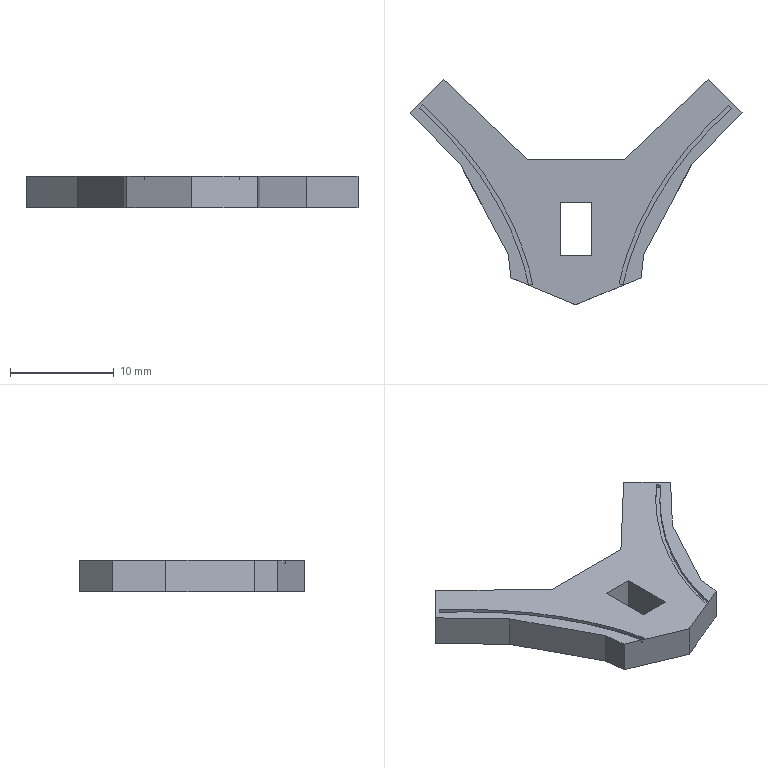Part | SolidWorks | features BaseBody 1 | 1 solid | 29 faces | box 31.951 x 21.72 x 3 mm | volume 821.926 mm3 | plane 25 | spline 4
STEP:
#1=CARTESIAN_POINT('',(13.317,21.551,1.2));
#2=VERTEX_POINT('',#1);
#3=CARTESIAN_POINT('',(2.742,4.389,1.2));
#4=VERTEX_POINT('',#3);
#5=CARTESIAN_POINT('',(13.317,21.551,1.2));
#6=CARTESIAN_POINT('',(10.685,19.267,1.2));
#7=CARTESIAN_POINT('',(4.586,13.173,1.2));
#8=CARTESIAN_POINT('',(2.742,4.389,1.2));
#9=B_SPLINE_CURVE_WITH_KNOTS('',3,(#5,#6,#7,#8),.UNSPECIFIED.,.F.,.F.,(4,4),(0.211,0.9451),.UNSPECIFIED.);
#10=EDGE_CURVE('',#2,#4,#9,.T.);
#11=ORIENTED_EDGE('',*,*,#10,.T.);
#12=CARTESIAN_POINT('',(3.133,4.307,1.2));
#13=VERTEX_POINT('',#12);
#14=CARTESIAN_POINT('',(3.133,4.307,1.2));
#15=DIRECTION('',(-0.9787,0.2054,0.));
#16=VECTOR('',#15,1000.);
#17=LINE('',#14,#16);
#18=EDGE_CURVE('',#13,#4,#17,.T.);
#19=ORIENTED_EDGE('',*,*,#18,.F.);
#20=CARTESIAN_POINT('',(13.579,21.248,1.2));
#21=VERTEX_POINT('',#20);
#22=CARTESIAN_POINT('',(13.579,21.248,1.2));
#23=CARTESIAN_POINT('',(12.281,20.122,1.2));
#24=CARTESIAN_POINT('',(10.119,18.048,1.2));
#25=CARTESIAN_POINT('',(5.999,12.301,1.2));
#26=CARTESIAN_POINT('',(4.041,8.63,1.2));
#27=CARTESIAN_POINT('',(3.133,4.307,1.2));
#28=B_SPLINE_CURVE_WITH_KNOTS('',3,(#22,#23,#24,#25,#26,#27),.UNSPECIFIED.,.F.,.F.,(4,2,4),(0.,0.5,1.),.UNSPECIFIED.);
#29=EDGE_CURVE('',#21,#13,#28,.T.);
#30=ORIENTED_EDGE('',*,*,#29,.F.);
#31=CARTESIAN_POINT('',(13.317,21.551,1.2));
#32=DIRECTION('',(0.6554,-0.7553,0.));
#33=VECTOR('',#32,1000.);
#34=LINE('',#31,#33);
#35=EDGE_CURVE('',#2,#21,#34,.T.);
#36=ORIENTED_EDGE('',*,*,#35,.F.);
#37=EDGE_LOOP('',(#11,#19,#30,#36));
#38=FACE_OUTER_BOUND('',#37,.T.);
#39=CARTESIAN_POINT('',(7.734,15.408,1.2));
#40=DIRECTION('',(0.,0.,-1.));
#41=DIRECTION('',(0.,-1.,0.));
#42=AXIS2_PLACEMENT_3D('',#39,#40,#41);
#43=PLANE('',#42);
#44=ADVANCED_FACE('',(#38),#43,.F.);
#45=CARTESIAN_POINT('',(3.133,4.307,1.5));
#46=VERTEX_POINT('',#45);
#47=CARTESIAN_POINT('',(2.742,4.389,1.5));
#48=VERTEX_POINT('',#47);
#49=CARTESIAN_POINT('',(3.133,4.307,1.5));
#50=DIRECTION('',(-0.9787,0.2054,0.));
#51=VECTOR('',#50,1000.);
#52=LINE('',#49,#51);
#53=EDGE_CURVE('',#46,#48,#52,.T.);
#54=ORIENTED_EDGE('',*,*,#53,.F.);
#55=CARTESIAN_POINT('',(3.133,4.307,1.2));
#56=DIRECTION('',(0.,0.,1.));
#57=VECTOR('',#56,1000.);
#58=LINE('',#55,#57);
#59=EDGE_CURVE('',#13,#46,#58,.T.);
#60=ORIENTED_EDGE('',*,*,#59,.F.);
#61=ORIENTED_EDGE('',*,*,#18,.T.);
#62=CARTESIAN_POINT('',(2.742,4.389,1.2));
#63=DIRECTION('',(0.,0.,1.));
#64=VECTOR('',#63,1000.);
#65=LINE('',#62,#64);
#66=EDGE_CURVE('',#4,#48,#65,.T.);
#67=ORIENTED_EDGE('',*,*,#66,.T.);
#68=EDGE_LOOP('',(#54,#60,#61,#67));
#69=FACE_OUTER_BOUND('',#68,.T.);
#70=CARTESIAN_POINT('',(3.133,4.307,1.2));
#71=DIRECTION('',(0.2054,0.9787,0.));
#72=DIRECTION('',(0.,0.,-1.));
#73=AXIS2_PLACEMENT_3D('',#70,#71,#72);
#74=PLANE('',#73);
#75=ADVANCED_FACE('',(#69),#74,.T.);
#76=CARTESIAN_POINT('',(13.579,21.248,1.5));
#77=VERTEX_POINT('',#76);
#78=CARTESIAN_POINT('',(13.579,21.248,1.5));
#79=CARTESIAN_POINT('',(12.281,20.122,1.5));
#80=CARTESIAN_POINT('',(10.119,18.048,1.5));
#81=CARTESIAN_POINT('',(5.999,12.301,1.5));
#82=CARTESIAN_POINT('',(4.041,8.63,1.5));
#83=CARTESIAN_POINT('',(3.133,4.307,1.5));
#84=B_SPLINE_CURVE_WITH_KNOTS('',3,(#78,#79,#80,#81,#82,#83),.UNSPECIFIED.,.F.,.F.,(4,2,4),(0.,0.5,1.),.UNSPECIFIED.);
#85=EDGE_CURVE('',#77,#46,#84,.T.);
#86=ORIENTED_EDGE('',*,*,#85,.F.);
#87=CARTESIAN_POINT('',(13.579,21.248,1.2));
#88=DIRECTION('',(0.,0.,1.));
#89=VECTOR('',#88,1000.);
#90=LINE('',#87,#89);
#91=EDGE_CURVE('',#21,#77,#90,.T.);
#92=ORIENTED_EDGE('',*,*,#91,.F.);
#93=ORIENTED_EDGE('',*,*,#29,.T.);
#94=ORIENTED_EDGE('',*,*,#59,.T.);
#95=EDGE_LOOP('',(#86,#92,#93,#94));
#96=FACE_OUTER_BOUND('',#95,.T.);
#97=CARTESIAN_POINT('',(13.579,21.248,1.2));
#98=CARTESIAN_POINT('',(13.579,21.248,1.5));
#99=CARTESIAN_POINT('',(12.281,20.122,1.2));
#100=CARTESIAN_POINT('',(12.281,20.122,1.5));
#101=CARTESIAN_POINT('',(10.119,18.048,1.2));
#102=CARTESIAN_POINT('',(10.119,18.048,1.5));
#103=CARTESIAN_POINT('',(5.999,12.301,1.2));
#104=CARTESIAN_POINT('',(5.999,12.301,1.5));
#105=CARTESIAN_POINT('',(4.041,8.63,1.2));
#106=CARTESIAN_POINT('',(4.041,8.63,1.5));
#107=CARTESIAN_POINT('',(3.133,4.307,1.2));
#108=CARTESIAN_POINT('',(3.133,4.307,1.5));
#109=B_SPLINE_SURFACE_WITH_KNOTS('',3,1,((#97,#98),(#99,#100),(#101,#102),(#103,#104),(#105,#106),(#107,#108)),.UNSPECIFIED.,.F.,.F.,.F.,(4,2,4),(2,2),(0.,0.5,1.),(0.,1.),.UNSPECIFIED.);
#110=ADVANCED_FACE('',(#96),#109,.T.);
#111=CARTESIAN_POINT('',(13.317,21.551,1.5));
#112=VERTEX_POINT('',#111);
#113=CARTESIAN_POINT('',(13.317,21.551,1.5));
#114=DIRECTION('',(0.6554,-0.7553,0.));
#115=VECTOR('',#114,1000.);
#116=LINE('',#113,#115);
#117=EDGE_CURVE('',#112,#77,#116,.T.);
#118=ORIENTED_EDGE('',*,*,#117,.F.);
#119=CARTESIAN_POINT('',(13.317,21.551,1.2));
#120=DIRECTION('',(0.,0.,1.));
#121=VECTOR('',#120,1000.);
#122=LINE('',#119,#121);
#123=EDGE_CURVE('',#2,#112,#122,.T.);
#124=ORIENTED_EDGE('',*,*,#123,.F.);
#125=ORIENTED_EDGE('',*,*,#35,.T.);
#126=ORIENTED_EDGE('',*,*,#91,.T.);
#127=EDGE_LOOP('',(#118,#124,#125,#126));
#128=FACE_OUTER_BOUND('',#127,.T.);
#129=CARTESIAN_POINT('',(13.317,21.551,1.2));
#130=DIRECTION('',(-0.7553,-0.6554,0.));
#131=DIRECTION('',(-0.6554,0.7553,0.));
#132=AXIS2_PLACEMENT_3D('',#129,#130,#131);
#133=PLANE('',#132);
#134=ADVANCED_FACE('',(#128),#133,.T.);
#135=CARTESIAN_POINT('',(13.317,21.551,1.5));
#136=CARTESIAN_POINT('',(10.685,19.267,1.5));
#137=CARTESIAN_POINT('',(4.586,13.173,1.5));
#138=CARTESIAN_POINT('',(2.742,4.389,1.5));
#139=B_SPLINE_CURVE_WITH_KNOTS('',3,(#135,#136,#137,#138),.UNSPECIFIED.,.F.,.F.,(4,4),(0.211,0.9451),.UNSPECIFIED.);
#140=EDGE_CURVE('',#112,#48,#139,.T.);
#141=ORIENTED_EDGE('',*,*,#140,.T.);
#142=ORIENTED_EDGE('',*,*,#66,.F.);
#143=ORIENTED_EDGE('',*,*,#10,.F.);
#144=ORIENTED_EDGE('',*,*,#123,.T.);
#145=EDGE_LOOP('',(#141,#142,#143,#144));
#146=FACE_OUTER_BOUND('',#145,.T.);
#147=CARTESIAN_POINT('',(13.317,21.551,1.2));
#148=CARTESIAN_POINT('',(13.317,21.551,1.5));
#149=CARTESIAN_POINT('',(10.685,19.267,1.2));
#150=CARTESIAN_POINT('',(10.685,19.267,1.5));
#151=CARTESIAN_POINT('',(4.586,13.173,1.2));
#152=CARTESIAN_POINT('',(4.586,13.173,1.5));
#153=CARTESIAN_POINT('',(2.742,4.389,1.2));
#154=CARTESIAN_POINT('',(2.742,4.389,1.5));
#155=B_SPLINE_SURFACE_WITH_KNOTS('',3,1,((#147,#148),(#149,#150),(#151,#152),(#153,#154)),.UNSPECIFIED.,.F.,.F.,.F.,(4,4),(2,2),(0.211,0.9451),(0.,1.),.UNSPECIFIED.);
#156=ADVANCED_FACE('',(#146),#155,.F.);
#157=CARTESIAN_POINT('',(-16.223,21.611,1.5));
#158=VERTEX_POINT('',#157);
#159=CARTESIAN_POINT('',(-5.569,4.343,1.5));
#160=VERTEX_POINT('',#159);
#161=CARTESIAN_POINT('',(-16.223,21.611,1.5));
#162=CARTESIAN_POINT('',(-13.627,19.373,1.5));
#163=CARTESIAN_POINT('',(-7.418,13.231,1.5));
#164=CARTESIAN_POINT('',(-5.569,4.343,1.5));
#165=B_SPLINE_CURVE_WITH_KNOTS('',3,(#161,#162,#163,#164),.UNSPECIFIED.,.F.,.F.,(4,4),(0.2044,0.9463),.UNSPECIFIED.);
#166=EDGE_CURVE('',#158,#160,#165,.T.);
#167=ORIENTED_EDGE('',*,*,#166,.F.);
#168=CARTESIAN_POINT('',(-16.223,21.611,1.2));
#169=VERTEX_POINT('',#168);
#170=CARTESIAN_POINT('',(-16.223,21.611,1.2));
#171=DIRECTION('',(0.,0.,1.));
#172=VECTOR('',#171,1000.);
#173=LINE('',#170,#172);
#174=EDGE_CURVE('',#169,#158,#173,.T.);
#175=ORIENTED_EDGE('',*,*,#174,.F.);
#176=CARTESIAN_POINT('',(-5.569,4.343,1.2));
#177=VERTEX_POINT('',#176);
#178=CARTESIAN_POINT('',(-16.223,21.611,1.2));
#179=CARTESIAN_POINT('',(-13.627,19.373,1.2));
#180=CARTESIAN_POINT('',(-7.418,13.231,1.2));
#181=CARTESIAN_POINT('',(-5.569,4.343,1.2));
#182=B_SPLINE_CURVE_WITH_KNOTS('',3,(#178,#179,#180,#181),.UNSPECIFIED.,.F.,.F.,(4,4),(0.2044,0.9463),.UNSPECIFIED.);
#183=EDGE_CURVE('',#169,#177,#182,.T.);
#184=ORIENTED_EDGE('',*,*,#183,.T.);
#185=CARTESIAN_POINT('',(-5.569,4.343,1.2));
#186=DIRECTION('',(0.,0.,1.));
#187=VECTOR('',#186,1000.);
#188=LINE('',#185,#187);
#189=EDGE_CURVE('',#177,#160,#188,.T.);
#190=ORIENTED_EDGE('',*,*,#189,.T.);
#191=EDGE_LOOP('',(#167,#175,#184,#190));
#192=FACE_OUTER_BOUND('',#191,.T.);
#193=CARTESIAN_POINT('',(-16.223,21.611,1.2));
#194=CARTESIAN_POINT('',(-16.223,21.611,1.5));
#195=CARTESIAN_POINT('',(-13.627,19.373,1.2));
#196=CARTESIAN_POINT('',(-13.627,19.373,1.5));
#197=CARTESIAN_POINT('',(-7.418,13.231,1.2));
#198=CARTESIAN_POINT('',(-7.418,13.231,1.5));
#199=CARTESIAN_POINT('',(-5.569,4.343,1.2));
#200=CARTESIAN_POINT('',(-5.569,4.343,1.5));
#201=B_SPLINE_SURFACE_WITH_KNOTS('',3,1,((#193,#194),(#195,#196),(#197,#198),(#199,#200)),.UNSPECIFIED.,.F.,.F.,.F.,(4,4),(2,2),(0.2044,0.9463),(0.,1.),.UNSPECIFIED.);
#202=ADVANCED_FACE('',(#192),#201,.T.);
#203=CARTESIAN_POINT('',(-16.484,21.308,1.5));
#204=VERTEX_POINT('',#203);
#205=CARTESIAN_POINT('',(-16.484,21.308,1.5));
#206=DIRECTION('',(0.6531,0.7573,0.));
#207=VECTOR('',#206,1000.);
#208=LINE('',#205,#207);
#209=EDGE_CURVE('',#204,#158,#208,.T.);
#210=ORIENTED_EDGE('',*,*,#209,.F.);
#211=CARTESIAN_POINT('',(-16.484,21.308,1.2));
#212=VERTEX_POINT('',#211);
#213=CARTESIAN_POINT('',(-16.484,21.308,1.2));
#214=DIRECTION('',(0.,0.,1.));
#215=VECTOR('',#214,1000.);
#216=LINE('',#213,#215);
#217=EDGE_CURVE('',#212,#204,#216,.T.);
#218=ORIENTED_EDGE('',*,*,#217,.F.);
#219=CARTESIAN_POINT('',(-16.484,21.308,1.2));
#220=DIRECTION('',(0.6531,0.7573,0.));
#221=VECTOR('',#220,1000.);
#222=LINE('',#219,#221);
#223=EDGE_CURVE('',#212,#169,#222,.T.);
#224=ORIENTED_EDGE('',*,*,#223,.T.);
#225=ORIENTED_EDGE('',*,*,#174,.T.);
#226=EDGE_LOOP('',(#210,#218,#224,#225));
#227=FACE_OUTER_BOUND('',#226,.T.);
#228=CARTESIAN_POINT('',(-16.484,21.308,1.2));
#229=DIRECTION('',(0.7573,-0.6531,0.));
#230=DIRECTION('',(0.,0.,-1.));
#231=AXIS2_PLACEMENT_3D('',#228,#229,#230);
#232=PLANE('',#231);
#233=ADVANCED_FACE('',(#227),#232,.T.);
#234=CARTESIAN_POINT('',(-5.963,4.271,1.2));
#235=VERTEX_POINT('',#234);
#236=CARTESIAN_POINT('',(-5.947,4.265,1.2));
#237=VERTEX_POINT('',#236);
#238=CARTESIAN_POINT('',(-1.413,2.373,1.2));
#239=DIRECTION('',(0.9229,-0.3851,0.));
#240=VECTOR('',#239,1000.);
#241=LINE('',#238,#240);
#242=EDGE_CURVE('',#235,#237,#241,.T.);
#243=ORIENTED_EDGE('',*,*,#242,.T.);
#244=CARTESIAN_POINT('',(-5.569,4.343,1.2));
#245=DIRECTION('',(-0.979,-0.2036,0.));
#246=VECTOR('',#245,1000.);
#247=LINE('',#244,#246);
#248=EDGE_CURVE('',#177,#237,#247,.T.);
#249=ORIENTED_EDGE('',*,*,#248,.F.);
#250=ORIENTED_EDGE('',*,*,#183,.F.);
#251=ORIENTED_EDGE('',*,*,#223,.F.);
#252=CARTESIAN_POINT('',(-16.484,21.308,1.2));
#253=CARTESIAN_POINT('',(-15.204,20.204,1.2));
#254=CARTESIAN_POINT('',(-13.024,18.13,1.2));
#255=CARTESIAN_POINT('',(-8.858,12.347,1.2));
#256=CARTESIAN_POINT('',(-6.874,8.642,1.2));
#257=CARTESIAN_POINT('',(-5.963,4.271,1.2));
#258=B_SPLINE_CURVE_WITH_KNOTS('',3,(#252,#253,#254,#255,#256,#257),.UNSPECIFIED.,.F.,.F.,(4,2,4),(0.,0.5,0.9996),.UNSPECIFIED.);
#259=EDGE_CURVE('',#212,#235,#258,.T.);
#260=ORIENTED_EDGE('',*,*,#259,.T.);
#261=EDGE_LOOP('',(#243,#249,#250,#251,#260));
#262=FACE_OUTER_BOUND('',#261,.T.);
#263=CARTESIAN_POINT('',(-10.94,15.237,1.2));
#264=DIRECTION('',(0.,0.,1.));
#265=DIRECTION('',(1.,0.,0.));
#266=AXIS2_PLACEMENT_3D('',#263,#264,#265);
#267=PLANE('',#266);
#268=ADVANCED_FACE('',(#262),#267,.T.);
#269=CARTESIAN_POINT('',(-5.947,4.265,1.5));
#270=VERTEX_POINT('',#269);
#271=CARTESIAN_POINT('',(-5.947,4.265,1.5));
#272=DIRECTION('',(0.,0.,1.));
#273=VECTOR('',#272,1000.);
#274=LINE('',#271,#273);
#275=EDGE_CURVE('',#237,#270,#274,.T.);
#276=ORIENTED_EDGE('',*,*,#275,.T.);
#277=CARTESIAN_POINT('',(-5.569,4.343,1.5));
#278=DIRECTION('',(-0.979,-0.2036,0.));
#279=VECTOR('',#278,1000.);
#280=LINE('',#277,#279);
#281=EDGE_CURVE('',#160,#270,#280,.T.);
#282=ORIENTED_EDGE('',*,*,#281,.F.);
#283=ORIENTED_EDGE('',*,*,#189,.F.);
#284=ORIENTED_EDGE('',*,*,#248,.T.);
#285=EDGE_LOOP('',(#276,#282,#283,#284));
#286=FACE_OUTER_BOUND('',#285,.T.);
#287=CARTESIAN_POINT('',(-5.569,4.343,1.2));
#288=DIRECTION('',(-0.2036,0.979,0.));
#289=DIRECTION('',(0.,0.,1.));
#290=AXIS2_PLACEMENT_3D('',#287,#288,#289);
#291=PLANE('',#290);
#292=ADVANCED_FACE('',(#286),#291,.T.);
#293=ORIENTED_EDGE('',*,*,#259,.F.);
#294=ORIENTED_EDGE('',*,*,#217,.T.);
#295=CARTESIAN_POINT('',(-5.963,4.271,1.5));
#296=VERTEX_POINT('',#295);
#297=CARTESIAN_POINT('',(-16.484,21.308,1.5));
#298=CARTESIAN_POINT('',(-15.204,20.204,1.5));
#299=CARTESIAN_POINT('',(-13.024,18.13,1.5));
#300=CARTESIAN_POINT('',(-8.858,12.347,1.5));
#301=CARTESIAN_POINT('',(-6.874,8.642,1.5));
#302=CARTESIAN_POINT('',(-5.963,4.271,1.5));
#303=B_SPLINE_CURVE_WITH_KNOTS('',3,(#297,#298,#299,#300,#301,#302),.UNSPECIFIED.,.F.,.F.,(4,2,4),(0.,0.5,0.9996),.UNSPECIFIED.);
#304=EDGE_CURVE('',#204,#296,#303,.T.);
#305=ORIENTED_EDGE('',*,*,#304,.T.);
#306=CARTESIAN_POINT('',(-5.963,4.271,1.2));
#307=DIRECTION('',(0.,0.,1.));
#308=VECTOR('',#307,1000.);
#309=LINE('',#306,#308);
#310=EDGE_CURVE('',#235,#296,#309,.T.);
#311=ORIENTED_EDGE('',*,*,#310,.F.);
#312=EDGE_LOOP('',(#293,#294,#305,#311));
#313=FACE_OUTER_BOUND('',#312,.T.);
#314=CARTESIAN_POINT('',(-16.484,21.308,1.2));
#315=CARTESIAN_POINT('',(-16.484,21.308,1.5));
#316=CARTESIAN_POINT('',(-15.204,20.204,1.2));
#317=CARTESIAN_POINT('',(-15.204,20.204,1.5));
#318=CARTESIAN_POINT('',(-13.024,18.13,1.2));
#319=CARTESIAN_POINT('',(-13.024,18.13,1.5));
#320=CARTESIAN_POINT('',(-8.858,12.347,1.2));
#321=CARTESIAN_POINT('',(-8.858,12.347,1.5));
#322=CARTESIAN_POINT('',(-6.874,8.642,1.2));
#323=CARTESIAN_POINT('',(-6.874,8.642,1.5));
#324=CARTESIAN_POINT('',(-5.963,4.271,1.2));
#325=CARTESIAN_POINT('',(-5.963,4.271,1.5));
#326=B_SPLINE_SURFACE_WITH_KNOTS('',3,1,((#314,#315),(#316,#317),(#318,#319),(#320,#321),(#322,#323),(#324,#325)),.UNSPECIFIED.,.F.,.F.,.F.,(4,2,4),(2,2),(0.,0.5,0.9996),(0.,1.),.UNSPECIFIED.);
#327=ADVANCED_FACE('',(#313),#326,.F.);
#328=CARTESIAN_POINT('',(0.0944,12.212,-1.5));
#329=VERTEX_POINT('',#328);
#330=CARTESIAN_POINT('',(-2.901,12.212,-1.5));
#331=VERTEX_POINT('',#330);
#332=CARTESIAN_POINT('',(0.0944,12.212,-1.5));
#333=DIRECTION('',(-1.,0.,0.));
#334=VECTOR('',#333,1000.);
#335=LINE('',#332,#334);
#336=EDGE_CURVE('',#329,#331,#335,.T.);
#337=ORIENTED_EDGE('',*,*,#336,.F.);
#338=CARTESIAN_POINT('',(0.0944,12.212,1.5));
#339=VERTEX_POINT('',#338);
#340=CARTESIAN_POINT('',(0.0944,12.212,1.5));
#341=DIRECTION('',(0.,0.,-1.));
#342=VECTOR('',#341,1000.);
#343=LINE('',#340,#342);
#344=EDGE_CURVE('',#339,#329,#343,.T.);
#345=ORIENTED_EDGE('',*,*,#344,.F.);
#346=CARTESIAN_POINT('',(-2.901,12.212,1.5));
#347=VERTEX_POINT('',#346);
#348=CARTESIAN_POINT('',(0.0944,12.212,1.5));
#349=DIRECTION('',(-1.,0.,0.));
#350=VECTOR('',#349,1000.);
#351=LINE('',#348,#350);
#352=EDGE_CURVE('',#339,#347,#351,.T.);
#353=ORIENTED_EDGE('',*,*,#352,.T.);
#354=CARTESIAN_POINT('',(-2.901,12.212,1.5));
#355=DIRECTION('',(0.,0.,-1.));
#356=VECTOR('',#355,1000.);
#357=LINE('',#354,#356);
#358=EDGE_CURVE('',#347,#331,#357,.T.);
#359=ORIENTED_EDGE('',*,*,#358,.T.);
#360=EDGE_LOOP('',(#337,#345,#353,#359));
#361=FACE_OUTER_BOUND('',#360,.T.);
#362=CARTESIAN_POINT('',(0.0944,12.212,1.5));
#363=DIRECTION('',(0.,-1.,0.));
#364=DIRECTION('',(0.,0.,-1.));
#365=AXIS2_PLACEMENT_3D('',#362,#363,#364);
#366=PLANE('',#365);
#367=ADVANCED_FACE('',(#361),#366,.T.);
#368=CARTESIAN_POINT('',(0.0944,7.154,-1.5));
#369=VERTEX_POINT('',#368);
#370=CARTESIAN_POINT('',(0.0944,7.154,-1.5));
#371=DIRECTION('',(0.,1.,0.));
#372=VECTOR('',#371,1000.);
#373=LINE('',#370,#372);
#374=EDGE_CURVE('',#369,#329,#373,.T.);
#375=ORIENTED_EDGE('',*,*,#374,.F.);
#376=CARTESIAN_POINT('',(0.0944,7.154,1.5));
#377=VERTEX_POINT('',#376);
#378=CARTESIAN_POINT('',(0.0944,7.154,1.5));
#379=DIRECTION('',(0.,0.,-1.));
#380=VECTOR('',#379,1000.);
#381=LINE('',#378,#380);
#382=EDGE_CURVE('',#377,#369,#381,.T.);
#383=ORIENTED_EDGE('',*,*,#382,.F.);
#384=CARTESIAN_POINT('',(0.0944,7.154,1.5));
#385=DIRECTION('',(0.,1.,0.));
#386=VECTOR('',#385,1000.);
#387=LINE('',#384,#386);
#388=EDGE_CURVE('',#377,#339,#387,.T.);
#389=ORIENTED_EDGE('',*,*,#388,.T.);
#390=ORIENTED_EDGE('',*,*,#344,.T.);
#391=EDGE_LOOP('',(#375,#383,#389,#390));
#392=FACE_OUTER_BOUND('',#391,.T.);
#393=CARTESIAN_POINT('',(0.0944,7.154,1.5));
#394=DIRECTION('',(-1.,0.,0.));
#395=DIRECTION('',(0.,0.,1.));
#396=AXIS2_PLACEMENT_3D('',#393,#394,#395);
#397=PLANE('',#396);
#398=ADVANCED_FACE('',(#392),#397,.T.);
#399=CARTESIAN_POINT('',(-2.901,7.154,-1.5));
#400=VERTEX_POINT('',#399);
#401=CARTESIAN_POINT('',(-2.901,7.154,-1.5));
#402=DIRECTION('',(1.,0.,0.));
#403=VECTOR('',#402,1000.);
#404=LINE('',#401,#403);
#405=EDGE_CURVE('',#400,#369,#404,.T.);
#406=ORIENTED_EDGE('',*,*,#405,.F.);
#407=CARTESIAN_POINT('',(-2.901,7.154,1.5));
#408=VERTEX_POINT('',#407);
#409=CARTESIAN_POINT('',(-2.901,7.154,1.5));
#410=DIRECTION('',(0.,0.,-1.));
#411=VECTOR('',#410,1000.);
#412=LINE('',#409,#411);
#413=EDGE_CURVE('',#408,#400,#412,.T.);
#414=ORIENTED_EDGE('',*,*,#413,.F.);
#415=CARTESIAN_POINT('',(-2.901,7.154,1.5));
#416=DIRECTION('',(1.,0.,0.));
#417=VECTOR('',#416,1000.);
#418=LINE('',#415,#417);
#419=EDGE_CURVE('',#408,#377,#418,.T.);
#420=ORIENTED_EDGE('',*,*,#419,.T.);
#421=ORIENTED_EDGE('',*,*,#382,.T.);
#422=EDGE_LOOP('',(#406,#414,#420,#421));
#423=FACE_OUTER_BOUND('',#422,.T.);
#424=CARTESIAN_POINT('',(-2.901,7.154,1.5));
#425=DIRECTION('',(0.,1.,0.));
#426=DIRECTION('',(1.,0.,0.));
#427=AXIS2_PLACEMENT_3D('',#424,#425,#426);
#428=PLANE('',#427);
#429=ADVANCED_FACE('',(#423),#428,.T.);
#430=CARTESIAN_POINT('',(-2.901,12.212,-1.5));
#431=DIRECTION('',(0.,-1.,0.));
#432=VECTOR('',#431,1000.);
#433=LINE('',#430,#432);
#434=EDGE_CURVE('',#331,#400,#433,.T.);
#435=ORIENTED_EDGE('',*,*,#434,.F.);
#436=ORIENTED_EDGE('',*,*,#358,.F.);
#437=CARTESIAN_POINT('',(-2.901,12.212,1.5));
#438=DIRECTION('',(0.,-1.,0.));
#439=VECTOR('',#438,1000.);
#440=LINE('',#437,#439);
#441=EDGE_CURVE('',#347,#408,#440,.T.);
#442=ORIENTED_EDGE('',*,*,#441,.T.);
#443=ORIENTED_EDGE('',*,*,#413,.T.);
#444=EDGE_LOOP('',(#435,#436,#442,#443));
#445=FACE_OUTER_BOUND('',#444,.T.);
#446=CARTESIAN_POINT('',(-2.901,12.212,1.5));
#447=DIRECTION('',(1.,0.,0.));
#448=DIRECTION('',(0.,1.,0.));
#449=AXIS2_PLACEMENT_3D('',#446,#447,#448);
#450=PLANE('',#449);
#451=ADVANCED_FACE('',(#445),#450,.T.);
#452=CARTESIAN_POINT('',(-7.916,7.257,-1.5));
#453=VERTEX_POINT('',#452);
#454=CARTESIAN_POINT('',(-7.669,4.983,-1.5));
#455=VERTEX_POINT('',#454);
#456=CARTESIAN_POINT('',(-7.669,4.983,-1.5));
#457=DIRECTION('',(0.108,-0.9941,0.));
#458=VECTOR('',#457,1000.);
#459=LINE('',#456,#458);
#460=EDGE_CURVE('',#453,#455,#459,.T.);
#461=ORIENTED_EDGE('',*,*,#460,.T.);
#462=CARTESIAN_POINT('',(-7.669,4.983,1.5));
#463=VERTEX_POINT('',#462);
#464=CARTESIAN_POINT('',(-7.669,4.983,1.5));
#465=DIRECTION('',(0.,0.,-1.));
#466=VECTOR('',#465,1000.);
#467=LINE('',#464,#466);
#468=EDGE_CURVE('',#463,#455,#467,.T.);
#469=ORIENTED_EDGE('',*,*,#468,.F.);
#470=CARTESIAN_POINT('',(-7.916,7.257,1.5));
#471=VERTEX_POINT('',#470);
#472=CARTESIAN_POINT('',(-7.669,4.983,1.5));
#473=DIRECTION('',(0.108,-0.9941,0.));
#474=VECTOR('',#473,1000.);
#475=LINE('',#472,#474);
#476=EDGE_CURVE('',#471,#463,#475,.T.);
#477=ORIENTED_EDGE('',*,*,#476,.F.);
#478=CARTESIAN_POINT('',(-7.916,7.257,1.5));
#479=DIRECTION('',(0.,0.,-1.));
#480=VECTOR('',#479,1000.);
#481=LINE('',#478,#480);
#482=EDGE_CURVE('',#471,#453,#481,.T.);
#483=ORIENTED_EDGE('',*,*,#482,.T.);
#484=EDGE_LOOP('',(#461,#469,#477,#483));
#485=FACE_OUTER_BOUND('',#484,.T.);
#486=CARTESIAN_POINT('',(-7.669,4.983,1.5));
#487=DIRECTION('',(0.9941,0.108,0.));
#488=DIRECTION('',(0.,0.,-1.));
#489=AXIS2_PLACEMENT_3D('',#486,#487,#488);
#490=PLANE('',#489);
#491=ADVANCED_FACE('',(#485),#490,.F.);
#492=CARTESIAN_POINT('',(-12.463,15.739,-1.5));
#493=VERTEX_POINT('',#492);
#494=CARTESIAN_POINT('',(-7.916,7.257,-1.5));
#495=DIRECTION('',(0.4725,-0.8813,0.));
#496=VECTOR('',#495,1000.);
#497=LINE('',#494,#496);
#498=EDGE_CURVE('',#493,#453,#497,.T.);
#499=ORIENTED_EDGE('',*,*,#498,.T.);
#500=ORIENTED_EDGE('',*,*,#482,.F.);
#501=CARTESIAN_POINT('',(-12.463,15.739,1.5));
#502=VERTEX_POINT('',#501);
#503=CARTESIAN_POINT('',(-7.916,7.257,1.5));
#504=DIRECTION('',(0.4725,-0.8813,0.));
#505=VECTOR('',#504,1000.);
#506=LINE('',#503,#505);
#507=EDGE_CURVE('',#502,#471,#506,.T.);
#508=ORIENTED_EDGE('',*,*,#507,.F.);
#509=CARTESIAN_POINT('',(-12.463,15.739,1.5));
#510=DIRECTION('',(0.,0.,-1.));
#511=VECTOR('',#510,1000.);
#512=LINE('',#509,#511);
#513=EDGE_CURVE('',#502,#493,#512,.T.);
#514=ORIENTED_EDGE('',*,*,#513,.T.);
#515=EDGE_LOOP('',(#499,#500,#508,#514));
#516=FACE_OUTER_BOUND('',#515,.T.);
#517=CARTESIAN_POINT('',(-7.916,7.257,1.5));
#518=DIRECTION('',(0.8813,0.4725,0.));
#519=DIRECTION('',(0.,0.,-1.));
#520=AXIS2_PLACEMENT_3D('',#517,#518,#519);
#521=PLANE('',#520);
#522=ADVANCED_FACE('',(#516),#521,.F.);
#523=CARTESIAN_POINT('',(-17.377,20.898,-1.5));
#524=VERTEX_POINT('',#523);
#525=CARTESIAN_POINT('',(-12.463,15.739,-1.5));
#526=DIRECTION('',(0.6897,-0.7241,0.));
#527=VECTOR('',#526,1000.);
#528=LINE('',#525,#527);
#529=EDGE_CURVE('',#524,#493,#528,.T.);
#530=ORIENTED_EDGE('',*,*,#529,.T.);
#531=ORIENTED_EDGE('',*,*,#513,.F.);
#532=CARTESIAN_POINT('',(-17.377,20.898,1.5));
#533=VERTEX_POINT('',#532);
#534=CARTESIAN_POINT('',(-12.463,15.739,1.5));
#535=DIRECTION('',(0.6897,-0.7241,0.));
#536=VECTOR('',#535,1000.);
#537=LINE('',#534,#536);
#538=EDGE_CURVE('',#533,#502,#537,.T.);
#539=ORIENTED_EDGE('',*,*,#538,.F.);
#540=CARTESIAN_POINT('',(-17.377,20.898,1.5));
#541=DIRECTION('',(0.,0.,-1.));
#542=VECTOR('',#541,1000.);
#543=LINE('',#540,#542);
#544=EDGE_CURVE('',#533,#524,#543,.T.);
#545=ORIENTED_EDGE('',*,*,#544,.T.);
#546=EDGE_LOOP('',(#530,#531,#539,#545));
#547=FACE_OUTER_BOUND('',#546,.T.);
#548=CARTESIAN_POINT('',(-12.463,15.739,1.5));
#549=DIRECTION('',(0.7241,0.6897,0.));
#550=DIRECTION('',(0.,0.,-1.));
#551=AXIS2_PLACEMENT_3D('',#548,#549,#550);
#552=PLANE('',#551);
#553=ADVANCED_FACE('',(#547),#552,.F.);
#554=CARTESIAN_POINT('',(-14.183,24.093,-1.5));
#555=VERTEX_POINT('',#554);
#556=CARTESIAN_POINT('',(-17.377,20.898,-1.5));
#557=DIRECTION('',(-0.707,-0.7073,0.));
#558=VECTOR('',#557,1000.);
#559=LINE('',#556,#558);
#560=EDGE_CURVE('',#555,#524,#559,.T.);
#561=ORIENTED_EDGE('',*,*,#560,.T.);
#562=ORIENTED_EDGE('',*,*,#544,.F.);
#563=CARTESIAN_POINT('',(-14.183,24.093,1.5));
#564=VERTEX_POINT('',#563);
#565=CARTESIAN_POINT('',(-17.377,20.898,1.5));
#566=DIRECTION('',(-0.707,-0.7073,0.));
#567=VECTOR('',#566,1000.);
#568=LINE('',#565,#567);
#569=EDGE_CURVE('',#564,#533,#568,.T.);
#570=ORIENTED_EDGE('',*,*,#569,.F.);
#571=CARTESIAN_POINT('',(-14.183,24.093,1.5));
#572=DIRECTION('',(0.,0.,-1.));
#573=VECTOR('',#572,1000.);
#574=LINE('',#571,#573);
#575=EDGE_CURVE('',#564,#555,#574,.T.);
#576=ORIENTED_EDGE('',*,*,#575,.T.);
#577=EDGE_LOOP('',(#561,#562,#570,#576));
#578=FACE_OUTER_BOUND('',#577,.T.);
#579=CARTESIAN_POINT('',(-17.377,20.898,1.5));
#580=DIRECTION('',(0.7073,-0.707,0.));
#581=DIRECTION('',(0.,0.,-1.));
#582=AXIS2_PLACEMENT_3D('',#579,#580,#581);
#583=PLANE('',#582);
#584=ADVANCED_FACE('',(#578),#583,.F.);
#585=CARTESIAN_POINT('',(-6.071,16.351,-1.5));
#586=VERTEX_POINT('',#585);
#587=CARTESIAN_POINT('',(-14.183,24.093,-1.5));
#588=DIRECTION('',(-0.7234,0.6904,0.));
#589=VECTOR('',#588,1000.);
#590=LINE('',#587,#589);
#591=EDGE_CURVE('',#586,#555,#590,.T.);
#592=ORIENTED_EDGE('',*,*,#591,.T.);
#593=ORIENTED_EDGE('',*,*,#575,.F.);
#594=CARTESIAN_POINT('',(-6.071,16.351,1.5));
#595=VERTEX_POINT('',#594);
#596=CARTESIAN_POINT('',(-14.183,24.093,1.5));
#597=DIRECTION('',(-0.7234,0.6904,0.));
#598=VECTOR('',#597,1000.);
#599=LINE('',#596,#598);
#600=EDGE_CURVE('',#595,#564,#599,.T.);
#601=ORIENTED_EDGE('',*,*,#600,.F.);
#602=CARTESIAN_POINT('',(-6.071,16.351,1.5));
#603=DIRECTION('',(0.,0.,-1.));
#604=VECTOR('',#603,1000.);
#605=LINE('',#602,#604);
#606=EDGE_CURVE('',#595,#586,#605,.T.);
#607=ORIENTED_EDGE('',*,*,#606,.T.);
#608=EDGE_LOOP('',(#592,#593,#601,#607));
#609=FACE_OUTER_BOUND('',#608,.T.);
#610=CARTESIAN_POINT('',(-14.183,24.093,1.5));
#611=DIRECTION('',(-0.6904,-0.7234,0.));
#612=DIRECTION('',(-0.7234,0.6904,0.));
#613=AXIS2_PLACEMENT_3D('',#610,#611,#612);
#614=PLANE('',#613);
#615=ADVANCED_FACE('',(#609),#614,.F.);
#616=CARTESIAN_POINT('',(3.266,16.351,-1.5));
#617=VERTEX_POINT('',#616);
#618=CARTESIAN_POINT('',(-6.071,16.351,-1.5));
#619=DIRECTION('',(-1.,0.,0.));
#620=VECTOR('',#619,1000.);
#621=LINE('',#618,#620);
#622=EDGE_CURVE('',#617,#586,#621,.T.);
#623=ORIENTED_EDGE('',*,*,#622,.T.);
#624=ORIENTED_EDGE('',*,*,#606,.F.);
#625=CARTESIAN_POINT('',(3.266,16.351,1.5));
#626=VERTEX_POINT('',#625);
#627=CARTESIAN_POINT('',(-6.071,16.351,1.5));
#628=DIRECTION('',(-1.,0.,0.));
#629=VECTOR('',#628,1000.);
#630=LINE('',#627,#629);
#631=EDGE_CURVE('',#626,#595,#630,.T.);
#632=ORIENTED_EDGE('',*,*,#631,.F.);
#633=CARTESIAN_POINT('',(3.266,16.351,1.5));
#634=DIRECTION('',(0.,0.,-1.));
#635=VECTOR('',#634,1000.);
#636=LINE('',#633,#635);
#637=EDGE_CURVE('',#626,#617,#636,.T.);
#638=ORIENTED_EDGE('',*,*,#637,.T.);
#639=EDGE_LOOP('',(#623,#624,#632,#638));
#640=FACE_OUTER_BOUND('',#639,.T.);
#641=CARTESIAN_POINT('',(-6.071,16.351,1.5));
#642=DIRECTION('',(0.,-1.,0.));
#643=DIRECTION('',(0.,0.,-1.));
#644=AXIS2_PLACEMENT_3D('',#641,#642,#643);
#645=PLANE('',#644);
#646=ADVANCED_FACE('',(#640),#645,.F.);
#647=CARTESIAN_POINT('',(11.377,24.093,-1.5));
#648=VERTEX_POINT('',#647);
#649=CARTESIAN_POINT('',(3.266,16.351,-1.5));
#650=DIRECTION('',(-0.7234,-0.6905,0.));
#651=VECTOR('',#650,1000.);
#652=LINE('',#649,#651);
#653=EDGE_CURVE('',#648,#617,#652,.T.);
#654=ORIENTED_EDGE('',*,*,#653,.T.);
#655=ORIENTED_EDGE('',*,*,#637,.F.);
#656=CARTESIAN_POINT('',(11.377,24.093,1.5));
#657=VERTEX_POINT('',#656);
#658=CARTESIAN_POINT('',(3.266,16.351,1.5));
#659=DIRECTION('',(-0.7234,-0.6905,0.));
#660=VECTOR('',#659,1000.);
#661=LINE('',#658,#660);
#662=EDGE_CURVE('',#657,#626,#661,.T.);
#663=ORIENTED_EDGE('',*,*,#662,.F.);
#664=CARTESIAN_POINT('',(11.377,24.093,1.5));
#665=DIRECTION('',(0.,0.,-1.));
#666=VECTOR('',#665,1000.);
#667=LINE('',#664,#666);
#668=EDGE_CURVE('',#657,#648,#667,.T.);
#669=ORIENTED_EDGE('',*,*,#668,.T.);
#670=EDGE_LOOP('',(#654,#655,#663,#669));
#671=FACE_OUTER_BOUND('',#670,.T.);
#672=CARTESIAN_POINT('',(3.266,16.351,1.5));
#673=DIRECTION('',(0.6905,-0.7234,0.));
#674=DIRECTION('',(0.,0.,-1.));
#675=AXIS2_PLACEMENT_3D('',#672,#673,#674);
#676=PLANE('',#675);
#677=ADVANCED_FACE('',(#671),#676,.F.);
#678=CARTESIAN_POINT('',(14.573,20.899,-1.5));
#679=VERTEX_POINT('',#678);
#680=CARTESIAN_POINT('',(11.377,24.093,-1.5));
#681=DIRECTION('',(-0.7073,0.7069,0.));
#682=VECTOR('',#681,1000.);
#683=LINE('',#680,#682);
#684=EDGE_CURVE('',#679,#648,#683,.T.);
#685=ORIENTED_EDGE('',*,*,#684,.T.);
#686=ORIENTED_EDGE('',*,*,#668,.F.);
#687=CARTESIAN_POINT('',(14.573,20.899,1.5));
#688=VERTEX_POINT('',#687);
#689=CARTESIAN_POINT('',(11.377,24.093,1.5));
#690=DIRECTION('',(-0.7073,0.7069,0.));
#691=VECTOR('',#690,1000.);
#692=LINE('',#689,#691);
#693=EDGE_CURVE('',#688,#657,#692,.T.);
#694=ORIENTED_EDGE('',*,*,#693,.F.);
#695=CARTESIAN_POINT('',(14.573,20.899,1.5));
#696=DIRECTION('',(0.,0.,-1.));
#697=VECTOR('',#696,1000.);
#698=LINE('',#695,#697);
#699=EDGE_CURVE('',#688,#679,#698,.T.);
#700=ORIENTED_EDGE('',*,*,#699,.T.);
#701=EDGE_LOOP('',(#685,#686,#694,#700));
#702=FACE_OUTER_BOUND('',#701,.T.);
#703=CARTESIAN_POINT('',(11.377,24.093,1.5));
#704=DIRECTION('',(-0.7069,-0.7073,0.));
#705=DIRECTION('',(-0.7073,0.7069,0.));
#706=AXIS2_PLACEMENT_3D('',#703,#704,#705);
#707=PLANE('',#706);
#708=ADVANCED_FACE('',(#702),#707,.F.);
#709=CARTESIAN_POINT('',(9.657,15.736,-1.5));
#710=VERTEX_POINT('',#709);
#711=CARTESIAN_POINT('',(14.573,20.899,-1.5));
#712=DIRECTION('',(0.6896,0.7242,0.));
#713=VECTOR('',#712,1000.);
#714=LINE('',#711,#713);
#715=EDGE_CURVE('',#710,#679,#714,.T.);
#716=ORIENTED_EDGE('',*,*,#715,.T.);
#717=ORIENTED_EDGE('',*,*,#699,.F.);
#718=CARTESIAN_POINT('',(9.657,15.736,1.5));
#719=VERTEX_POINT('',#718);
#720=CARTESIAN_POINT('',(14.573,20.899,1.5));
#721=DIRECTION('',(0.6896,0.7242,0.));
#722=VECTOR('',#721,1000.);
#723=LINE('',#720,#722);
#724=EDGE_CURVE('',#719,#688,#723,.T.);
#725=ORIENTED_EDGE('',*,*,#724,.F.);
#726=CARTESIAN_POINT('',(9.657,15.736,1.5));
#727=DIRECTION('',(0.,0.,-1.));
#728=VECTOR('',#727,1000.);
#729=LINE('',#726,#728);
#730=EDGE_CURVE('',#719,#710,#729,.T.);
#731=ORIENTED_EDGE('',*,*,#730,.T.);
#732=EDGE_LOOP('',(#716,#717,#725,#731));
#733=FACE_OUTER_BOUND('',#732,.T.);
#734=CARTESIAN_POINT('',(14.573,20.899,1.5));
#735=DIRECTION('',(-0.7242,0.6896,0.));
#736=DIRECTION('',(0.,0.,1.));
#737=AXIS2_PLACEMENT_3D('',#734,#735,#736);
#738=PLANE('',#737);
#739=ADVANCED_FACE('',(#733),#738,.F.);
#740=CARTESIAN_POINT('',(5.111,7.256,-1.5));
#741=VERTEX_POINT('',#740);
#742=CARTESIAN_POINT('',(9.657,15.736,-1.5));
#743=DIRECTION('',(0.4724,0.8814,0.));
#744=VECTOR('',#743,1000.);
#745=LINE('',#742,#744);
#746=EDGE_CURVE('',#741,#710,#745,.T.);
#747=ORIENTED_EDGE('',*,*,#746,.T.);
#748=ORIENTED_EDGE('',*,*,#730,.F.);
#749=CARTESIAN_POINT('',(5.111,7.256,1.5));
#750=VERTEX_POINT('',#749);
#751=CARTESIAN_POINT('',(9.657,15.736,1.5));
#752=DIRECTION('',(0.4724,0.8814,0.));
#753=VECTOR('',#752,1000.);
#754=LINE('',#751,#753);
#755=EDGE_CURVE('',#750,#719,#754,.T.);
#756=ORIENTED_EDGE('',*,*,#755,.F.);
#757=CARTESIAN_POINT('',(5.111,7.256,1.5));
#758=DIRECTION('',(0.,0.,-1.));
#759=VECTOR('',#758,1000.);
#760=LINE('',#757,#759);
#761=EDGE_CURVE('',#750,#741,#760,.T.);
#762=ORIENTED_EDGE('',*,*,#761,.T.);
#763=EDGE_LOOP('',(#747,#748,#756,#762));
#764=FACE_OUTER_BOUND('',#763,.T.);
#765=CARTESIAN_POINT('',(9.657,15.736,1.5));
#766=DIRECTION('',(-0.8814,0.4724,0.));
#767=DIRECTION('',(0.,0.,1.));
#768=AXIS2_PLACEMENT_3D('',#765,#766,#767);
#769=PLANE('',#768);
#770=ADVANCED_FACE('',(#764),#769,.F.);
#771=CARTESIAN_POINT('',(4.865,4.985,-1.5));
#772=VERTEX_POINT('',#771);
#773=CARTESIAN_POINT('',(5.111,7.256,-1.5));
#774=DIRECTION('',(0.1077,0.9942,0.));
#775=VECTOR('',#774,1000.);
#776=LINE('',#773,#775);
#777=EDGE_CURVE('',#772,#741,#776,.T.);
#778=ORIENTED_EDGE('',*,*,#777,.T.);
#779=ORIENTED_EDGE('',*,*,#761,.F.);
#780=CARTESIAN_POINT('',(4.865,4.985,1.5));
#781=VERTEX_POINT('',#780);
#782=CARTESIAN_POINT('',(5.111,7.256,1.5));
#783=DIRECTION('',(0.1077,0.9942,0.));
#784=VECTOR('',#783,1000.);
#785=LINE('',#782,#784);
#786=EDGE_CURVE('',#781,#750,#785,.T.);
#787=ORIENTED_EDGE('',*,*,#786,.F.);
#788=CARTESIAN_POINT('',(4.865,4.985,1.5));
#789=DIRECTION('',(0.,0.,-1.));
#790=VECTOR('',#789,1000.);
#791=LINE('',#788,#790);
#792=EDGE_CURVE('',#781,#772,#791,.T.);
#793=ORIENTED_EDGE('',*,*,#792,.T.);
#794=EDGE_LOOP('',(#778,#779,#787,#793));
#795=FACE_OUTER_BOUND('',#794,.T.);
#796=CARTESIAN_POINT('',(5.111,7.256,1.5));
#797=DIRECTION('',(-0.9942,0.1077,0.));
#798=DIRECTION('',(0.,0.,1.));
#799=AXIS2_PLACEMENT_3D('',#796,#797,#798);
#800=PLANE('',#799);
#801=ADVANCED_FACE('',(#795),#800,.F.);
#802=CARTESIAN_POINT('',(-1.413,2.373,-1.5));
#803=VERTEX_POINT('',#802);
#804=CARTESIAN_POINT('',(4.865,4.985,-1.5));
#805=DIRECTION('',(0.9233,0.3841,0.));
#806=VECTOR('',#805,1000.);
#807=LINE('',#804,#806);
#808=EDGE_CURVE('',#803,#772,#807,.T.);
#809=ORIENTED_EDGE('',*,*,#808,.T.);
#810=ORIENTED_EDGE('',*,*,#792,.F.);
#811=CARTESIAN_POINT('',(-1.413,2.373,1.5));
#812=VERTEX_POINT('',#811);
#813=CARTESIAN_POINT('',(4.865,4.985,1.5));
#814=DIRECTION('',(0.9233,0.3841,0.));
#815=VECTOR('',#814,1000.);
#816=LINE('',#813,#815);
#817=EDGE_CURVE('',#812,#781,#816,.T.);
#818=ORIENTED_EDGE('',*,*,#817,.F.);
#819=CARTESIAN_POINT('',(-1.413,2.373,1.5));
#820=DIRECTION('',(0.,0.,-1.));
#821=VECTOR('',#820,1000.);
#822=LINE('',#819,#821);
#823=EDGE_CURVE('',#812,#803,#822,.T.);
#824=ORIENTED_EDGE('',*,*,#823,.T.);
#825=EDGE_LOOP('',(#809,#810,#818,#824));
#826=FACE_OUTER_BOUND('',#825,.T.);
#827=CARTESIAN_POINT('',(4.865,4.985,1.5));
#828=DIRECTION('',(-0.3841,0.9233,0.));
#829=DIRECTION('',(0.,0.,1.));
#830=AXIS2_PLACEMENT_3D('',#827,#828,#829);
#831=PLANE('',#830);
#832=ADVANCED_FACE('',(#826),#831,.F.);
#833=ORIENTED_EDGE('',*,*,#242,.F.);
#834=ORIENTED_EDGE('',*,*,#310,.T.);
#835=CARTESIAN_POINT('',(-1.413,2.373,1.5));
#836=DIRECTION('',(0.9229,-0.3851,0.));
#837=VECTOR('',#836,1000.);
#838=LINE('',#835,#837);
#839=EDGE_CURVE('',#463,#296,#838,.T.);
#840=ORIENTED_EDGE('',*,*,#839,.F.);
#841=ORIENTED_EDGE('',*,*,#468,.T.);
#842=CARTESIAN_POINT('',(-1.413,2.373,-1.5));
#843=DIRECTION('',(0.9229,-0.3851,0.));
#844=VECTOR('',#843,1000.);
#845=LINE('',#842,#844);
#846=EDGE_CURVE('',#455,#803,#845,.T.);
#847=ORIENTED_EDGE('',*,*,#846,.T.);
#848=ORIENTED_EDGE('',*,*,#823,.F.);
#849=CARTESIAN_POINT('',(-1.413,2.373,1.5));
#850=DIRECTION('',(0.9229,-0.3851,0.));
#851=VECTOR('',#850,1000.);
#852=LINE('',#849,#851);
#853=EDGE_CURVE('',#270,#812,#852,.T.);
#854=ORIENTED_EDGE('',*,*,#853,.F.);
#855=ORIENTED_EDGE('',*,*,#275,.F.);
#856=EDGE_LOOP('',(#833,#834,#840,#841,#847,#848,#854,#855));
#857=FACE_OUTER_BOUND('',#856,.T.);
#858=CARTESIAN_POINT('',(-1.413,2.373,1.5));
#859=DIRECTION('',(0.3851,0.9229,0.));
#860=DIRECTION('',(0.,0.,-1.));
#861=AXIS2_PLACEMENT_3D('',#858,#859,#860);
#862=PLANE('',#861);
#863=ADVANCED_FACE('',(#857),#862,.F.);
#864=ORIENTED_EDGE('',*,*,#434,.T.);
#865=ORIENTED_EDGE('',*,*,#405,.T.);
#866=ORIENTED_EDGE('',*,*,#374,.T.);
#867=ORIENTED_EDGE('',*,*,#336,.T.);
#868=EDGE_LOOP('',(#864,#865,#866,#867));
#869=FACE_BOUND('',#868,.T.);
#870=ORIENTED_EDGE('',*,*,#846,.F.);
#871=ORIENTED_EDGE('',*,*,#460,.F.);
#872=ORIENTED_EDGE('',*,*,#498,.F.);
#873=ORIENTED_EDGE('',*,*,#529,.F.);
#874=ORIENTED_EDGE('',*,*,#560,.F.);
#875=ORIENTED_EDGE('',*,*,#591,.F.);
#876=ORIENTED_EDGE('',*,*,#622,.F.);
#877=ORIENTED_EDGE('',*,*,#653,.F.);
#878=ORIENTED_EDGE('',*,*,#684,.F.);
#879=ORIENTED_EDGE('',*,*,#715,.F.);
#880=ORIENTED_EDGE('',*,*,#746,.F.);
#881=ORIENTED_EDGE('',*,*,#777,.F.);
#882=ORIENTED_EDGE('',*,*,#808,.F.);
#883=EDGE_LOOP('',(#870,#871,#872,#873,#874,#875,#876,#877,#878,#879,#880,#881,#882));
#884=FACE_OUTER_BOUND('',#883,.T.);
#885=CARTESIAN_POINT('',(0.,0.,-1.5));
#886=DIRECTION('',(0.,0.,1.));
#887=DIRECTION('',(1.,0.,0.));
#888=AXIS2_PLACEMENT_3D('',#885,#886,#887);
#889=PLANE('',#888);
#890=ADVANCED_FACE('',(#869,#884),#889,.F.);
#891=ORIENTED_EDGE('',*,*,#419,.F.);
#892=ORIENTED_EDGE('',*,*,#441,.F.);
#893=ORIENTED_EDGE('',*,*,#352,.F.);
#894=ORIENTED_EDGE('',*,*,#388,.F.);
#895=EDGE_LOOP('',(#891,#892,#893,#894));
#896=FACE_BOUND('',#895,.T.);
#897=ORIENTED_EDGE('',*,*,#140,.F.);
#898=ORIENTED_EDGE('',*,*,#117,.T.);
#899=ORIENTED_EDGE('',*,*,#85,.T.);
#900=ORIENTED_EDGE('',*,*,#53,.T.);
#901=EDGE_LOOP('',(#897,#898,#899,#900));
#902=FACE_BOUND('',#901,.T.);
#903=ORIENTED_EDGE('',*,*,#304,.F.);
#904=ORIENTED_EDGE('',*,*,#209,.T.);
#905=ORIENTED_EDGE('',*,*,#166,.T.);
#906=ORIENTED_EDGE('',*,*,#281,.T.);
#907=ORIENTED_EDGE('',*,*,#853,.T.);
#908=ORIENTED_EDGE('',*,*,#817,.T.);
#909=ORIENTED_EDGE('',*,*,#786,.T.);
#910=ORIENTED_EDGE('',*,*,#755,.T.);
#911=ORIENTED_EDGE('',*,*,#724,.T.);
#912=ORIENTED_EDGE('',*,*,#693,.T.);
#913=ORIENTED_EDGE('',*,*,#662,.T.);
#914=ORIENTED_EDGE('',*,*,#631,.T.);
#915=ORIENTED_EDGE('',*,*,#600,.T.);
#916=ORIENTED_EDGE('',*,*,#569,.T.);
#917=ORIENTED_EDGE('',*,*,#538,.T.);
#918=ORIENTED_EDGE('',*,*,#507,.T.);
#919=ORIENTED_EDGE('',*,*,#476,.T.);
#920=ORIENTED_EDGE('',*,*,#839,.T.);
#921=EDGE_LOOP('',(#903,#904,#905,#906,#907,#908,#909,#910,#911,#912,#913,#914,#915,#916,#917,#918,#919,#920));
#922=FACE_OUTER_BOUND('',#921,.T.);
#923=CARTESIAN_POINT('',(0.,0.,1.5));
#924=DIRECTION('',(0.,0.,1.));
#925=DIRECTION('',(1.,0.,0.));
#926=AXIS2_PLACEMENT_3D('',#923,#924,#925);
#927=PLANE('',#926);
#928=ADVANCED_FACE('',(#896,#902,#922),#927,.T.);
#929=CLOSED_SHELL('',(#44,#75,#110,#134,#156,#202,#233,#268,#292,#327,#367,#398,#429,#451,#491,#522,#553,#584,#615,#646,#677,#708,#739,#770,#801,#832,#863,#890,#928));
#930=MANIFOLD_SOLID_BREP('',#929);
#931=CARTESIAN_POINT('',(0.,0.,0.));
#932=DIRECTION('',(0.,0.,1.));
#933=DIRECTION('',(1.,0.,0.));
#934=AXIS2_PLACEMENT_3D('',#931,#932,#933);
#935=(LENGTH_UNIT()NAMED_UNIT(*)SI_UNIT(.MILLI.,.METRE.));
#936=UNCERTAINTY_MEASURE_WITH_UNIT(LENGTH_MEASURE(0.00001),#935,'','');
#937=(NAMED_UNIT(*)PLANE_ANGLE_UNIT()SI_UNIT($,.RADIAN.));
#938=(NAMED_UNIT(*)SI_UNIT($,.STERADIAN.)SOLID_ANGLE_UNIT());
#939=(GEOMETRIC_REPRESENTATION_CONTEXT(3)GLOBAL_UNCERTAINTY_ASSIGNED_CONTEXT((#936))GLOBAL_UNIT_ASSIGNED_CONTEXT((#935,#937,#938))REPRESENTATION_CONTEXT('',''));
#940=ADVANCED_BREP_SHAPE_REPRESENTATION('',(#930,#934),#939);